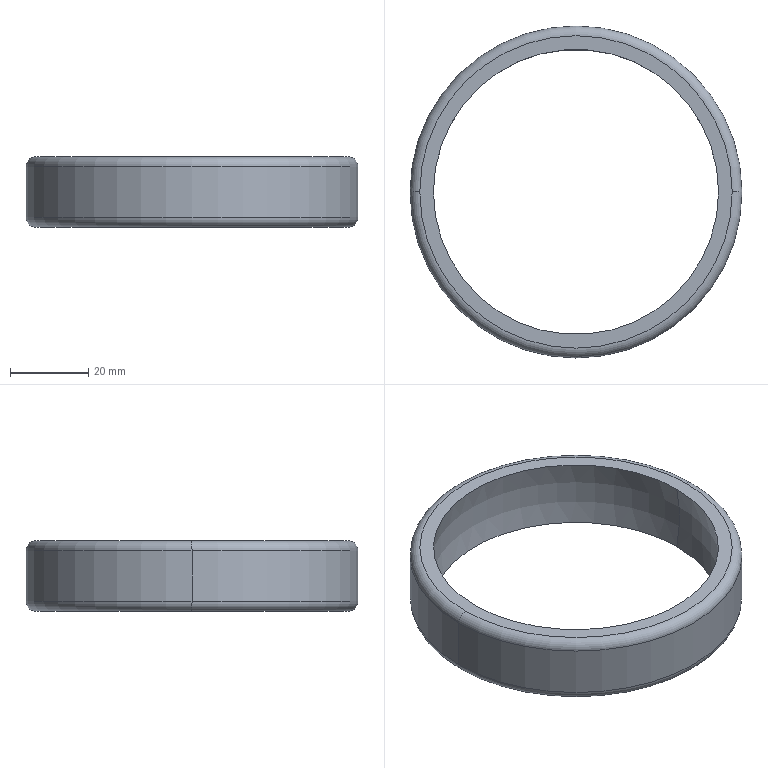Part | SolidWorks | features Extrusion 1, Fillet 1, RevCut 1 | 1 solid | 10 faces | box 85 x 85 x 18 mm | volume 23565 mm3 | torus 6 | cylinder 2 | plane 2 | commonest cylinder face diameters 85 x2
STEP:
#1=CARTESIAN_POINT('',(-40.,0.,-9.));
#2=VERTEX_POINT('',#1);
#3=CARTESIAN_POINT('',(40.,0.,-9.));
#4=VERTEX_POINT('',#3);
#5=CARTESIAN_POINT('',(0.,0.,-9.));
#6=DIRECTION('',(0.,0.,-1.));
#7=DIRECTION('',(1.,0.,0.));
#8=AXIS2_PLACEMENT_3D('',#5,#6,#7);
#9=CIRCLE('',#8,40.);
#10=EDGE_CURVE('',#2,#4,#9,.T.);
#11=ORIENTED_EDGE('',*,*,#10,.F.);
#12=CARTESIAN_POINT('',(-42.5,0.,-6.5));
#13=VERTEX_POINT('',#12);
#14=CARTESIAN_POINT('',(-40.,0.,-6.5));
#15=DIRECTION('',(0.,1.,0.));
#16=DIRECTION('',(-1.,0.,0.));
#17=AXIS2_PLACEMENT_3D('',#14,#15,#16);
#18=CIRCLE('',#17,2.5);
#19=EDGE_CURVE('',#2,#13,#18,.T.);
#20=ORIENTED_EDGE('',*,*,#19,.T.);
#21=CARTESIAN_POINT('',(42.5,0.,-6.5));
#22=VERTEX_POINT('',#21);
#23=CARTESIAN_POINT('',(0.,0.,-6.5));
#24=DIRECTION('',(0.,0.,1.));
#25=DIRECTION('',(1.,0.,0.));
#26=AXIS2_PLACEMENT_3D('',#23,#24,#25);
#27=CIRCLE('',#26,42.5);
#28=EDGE_CURVE('',#22,#13,#27,.T.);
#29=ORIENTED_EDGE('',*,*,#28,.F.);
#30=CARTESIAN_POINT('',(40.,0.,-6.5));
#31=DIRECTION('',(0.,-1.,0.));
#32=DIRECTION('',(0.,0.,-1.));
#33=AXIS2_PLACEMENT_3D('',#30,#31,#32);
#34=CIRCLE('',#33,2.5);
#35=EDGE_CURVE('',#4,#22,#34,.T.);
#36=ORIENTED_EDGE('',*,*,#35,.F.);
#37=EDGE_LOOP('',(#11,#20,#29,#36));
#38=FACE_OUTER_BOUND('',#37,.T.);
#39=CARTESIAN_POINT('',(0.,0.,-6.5));
#40=DIRECTION('',(0.,0.,1.));
#41=DIRECTION('',(1.,0.,0.));
#42=AXIS2_PLACEMENT_3D('',#39,#40,#41);
#43=TOROIDAL_SURFACE('',#42,40.,2.5);
#44=ADVANCED_FACE('',(#38),#43,.T.);
#45=CARTESIAN_POINT('',(-42.5,0.,6.5));
#46=VERTEX_POINT('',#45);
#47=CARTESIAN_POINT('',(42.5,0.,6.5));
#48=VERTEX_POINT('',#47);
#49=CARTESIAN_POINT('',(0.,0.,6.5));
#50=DIRECTION('',(0.,0.,-1.));
#51=DIRECTION('',(1.,0.,0.));
#52=AXIS2_PLACEMENT_3D('',#49,#50,#51);
#53=CIRCLE('',#52,42.5);
#54=EDGE_CURVE('',#46,#48,#53,.T.);
#55=ORIENTED_EDGE('',*,*,#54,.F.);
#56=CARTESIAN_POINT('',(-40.,0.,9.));
#57=VERTEX_POINT('',#56);
#58=CARTESIAN_POINT('',(-40.,0.,6.5));
#59=DIRECTION('',(0.,1.,0.));
#60=DIRECTION('',(-1.,0.,0.));
#61=AXIS2_PLACEMENT_3D('',#58,#59,#60);
#62=CIRCLE('',#61,2.5);
#63=EDGE_CURVE('',#46,#57,#62,.T.);
#64=ORIENTED_EDGE('',*,*,#63,.T.);
#65=CARTESIAN_POINT('',(40.,0.,9.));
#66=VERTEX_POINT('',#65);
#67=CARTESIAN_POINT('',(0.,0.,9.));
#68=DIRECTION('',(0.,0.,1.));
#69=DIRECTION('',(1.,0.,0.));
#70=AXIS2_PLACEMENT_3D('',#67,#68,#69);
#71=CIRCLE('',#70,40.);
#72=EDGE_CURVE('',#66,#57,#71,.T.);
#73=ORIENTED_EDGE('',*,*,#72,.F.);
#74=CARTESIAN_POINT('',(40.,0.,6.5));
#75=DIRECTION('',(0.,-1.,0.));
#76=DIRECTION('',(0.,0.,-1.));
#77=AXIS2_PLACEMENT_3D('',#74,#75,#76);
#78=CIRCLE('',#77,2.5);
#79=EDGE_CURVE('',#48,#66,#78,.T.);
#80=ORIENTED_EDGE('',*,*,#79,.F.);
#81=EDGE_LOOP('',(#55,#64,#73,#80));
#82=FACE_OUTER_BOUND('',#81,.T.);
#83=CARTESIAN_POINT('',(0.,0.,6.5));
#84=DIRECTION('',(0.,0.,1.));
#85=DIRECTION('',(1.,0.,0.));
#86=AXIS2_PLACEMENT_3D('',#83,#84,#85);
#87=TOROIDAL_SURFACE('',#86,40.,2.5);
#88=ADVANCED_FACE('',(#82),#87,.T.);
#89=CARTESIAN_POINT('',(36.5,0.,9.));
#90=VERTEX_POINT('',#89);
#91=CARTESIAN_POINT('',(-36.5,0.,9.));
#92=VERTEX_POINT('',#91);
#93=CARTESIAN_POINT('',(0.,0.,9.));
#94=DIRECTION('',(0.,0.,-1.));
#95=DIRECTION('',(-1.,0.,0.));
#96=AXIS2_PLACEMENT_3D('',#93,#94,#95);
#97=CIRCLE('',#96,36.5);
#98=EDGE_CURVE('',#90,#92,#97,.T.);
#99=ORIENTED_EDGE('',*,*,#98,.F.);
#100=CARTESIAN_POINT('',(36.5,0.,-9.));
#101=VERTEX_POINT('',#100);
#102=CARTESIAN_POINT('',(-7.591,0.,0.));
#103=DIRECTION('',(0.,1.,0.));
#104=DIRECTION('',(-1.,0.,0.));
#105=AXIS2_PLACEMENT_3D('',#102,#103,#104);
#106=CIRCLE('',#105,45.);
#107=EDGE_CURVE('',#90,#101,#106,.T.);
#108=ORIENTED_EDGE('',*,*,#107,.T.);
#109=CARTESIAN_POINT('',(-36.5,0.,-9.));
#110=VERTEX_POINT('',#109);
#111=CARTESIAN_POINT('',(0.,0.,-9.));
#112=DIRECTION('',(0.,0.,-1.));
#113=DIRECTION('',(-1.,0.,0.));
#114=AXIS2_PLACEMENT_3D('',#111,#112,#113);
#115=CIRCLE('',#114,36.5);
#116=EDGE_CURVE('',#101,#110,#115,.T.);
#117=ORIENTED_EDGE('',*,*,#116,.T.);
#118=CARTESIAN_POINT('',(7.591,0.,0.));
#119=DIRECTION('',(0.,-1.,0.));
#120=DIRECTION('',(0.,0.,-1.));
#121=AXIS2_PLACEMENT_3D('',#118,#119,#120);
#122=CIRCLE('',#121,45.);
#123=EDGE_CURVE('',#92,#110,#122,.T.);
#124=ORIENTED_EDGE('',*,*,#123,.F.);
#125=EDGE_LOOP('',(#99,#108,#117,#124));
#126=FACE_OUTER_BOUND('',#125,.T.);
#127=CARTESIAN_POINT('',(0.,0.,0.));
#128=DIRECTION('',(0.,0.,-1.));
#129=DIRECTION('',(-1.,0.,0.));
#130=AXIS2_PLACEMENT_3D('',#127,#128,#129);
#131=TOROIDAL_SURFACE('',#130,-7.591,45.);
#132=ADVANCED_FACE('',(#126),#131,.F.);
#133=ORIENTED_EDGE('',*,*,#54,.T.);
#134=CARTESIAN_POINT('',(42.5,0.,9.));
#135=DIRECTION('',(0.,0.,-1.));
#136=VECTOR('',#135,1000.);
#137=LINE('',#134,#136);
#138=EDGE_CURVE('',#48,#22,#137,.T.);
#139=ORIENTED_EDGE('',*,*,#138,.T.);
#140=ORIENTED_EDGE('',*,*,#28,.T.);
#141=CARTESIAN_POINT('',(-42.5,0.,9.));
#142=DIRECTION('',(0.,0.,-1.));
#143=VECTOR('',#142,1000.);
#144=LINE('',#141,#143);
#145=EDGE_CURVE('',#46,#13,#144,.T.);
#146=ORIENTED_EDGE('',*,*,#145,.F.);
#147=EDGE_LOOP('',(#133,#139,#140,#146));
#148=FACE_OUTER_BOUND('',#147,.T.);
#149=CARTESIAN_POINT('',(0.,0.,9.));
#150=DIRECTION('',(0.,0.,-1.));
#151=DIRECTION('',(-1.,0.,0.));
#152=AXIS2_PLACEMENT_3D('',#149,#150,#151);
#153=CYLINDRICAL_SURFACE('',#152,42.5);
#154=ADVANCED_FACE('',(#148),#153,.T.);
#155=ORIENTED_EDGE('',*,*,#72,.T.);
#156=CARTESIAN_POINT('',(0.,0.,9.));
#157=DIRECTION('',(0.,0.,1.));
#158=DIRECTION('',(1.,0.,0.));
#159=AXIS2_PLACEMENT_3D('',#156,#157,#158);
#160=CIRCLE('',#159,40.);
#161=EDGE_CURVE('',#57,#66,#160,.T.);
#162=ORIENTED_EDGE('',*,*,#161,.T.);
#163=EDGE_LOOP('',(#155,#162));
#164=FACE_OUTER_BOUND('',#163,.T.);
#165=CARTESIAN_POINT('',(0.,0.,9.));
#166=DIRECTION('',(0.,0.,-1.));
#167=DIRECTION('',(-1.,0.,0.));
#168=AXIS2_PLACEMENT_3D('',#165,#166,#167);
#169=CIRCLE('',#168,36.5);
#170=EDGE_CURVE('',#92,#90,#169,.T.);
#171=ORIENTED_EDGE('',*,*,#170,.T.);
#172=ORIENTED_EDGE('',*,*,#98,.T.);
#173=EDGE_LOOP('',(#171,#172));
#174=FACE_BOUND('',#173,.T.);
#175=CARTESIAN_POINT('',(0.,0.,9.));
#176=DIRECTION('',(0.,0.,1.));
#177=DIRECTION('',(1.,0.,0.));
#178=AXIS2_PLACEMENT_3D('',#175,#176,#177);
#179=PLANE('',#178);
#180=ADVANCED_FACE('',(#164,#174),#179,.T.);
#181=CARTESIAN_POINT('',(0.,0.,-9.));
#182=DIRECTION('',(0.,0.,-1.));
#183=DIRECTION('',(1.,0.,0.));
#184=AXIS2_PLACEMENT_3D('',#181,#182,#183);
#185=CIRCLE('',#184,40.);
#186=EDGE_CURVE('',#4,#2,#185,.T.);
#187=ORIENTED_EDGE('',*,*,#186,.T.);
#188=ORIENTED_EDGE('',*,*,#10,.T.);
#189=EDGE_LOOP('',(#187,#188));
#190=FACE_OUTER_BOUND('',#189,.T.);
#191=CARTESIAN_POINT('',(0.,0.,-9.));
#192=DIRECTION('',(0.,0.,-1.));
#193=DIRECTION('',(-1.,0.,0.));
#194=AXIS2_PLACEMENT_3D('',#191,#192,#193);
#195=CIRCLE('',#194,36.5);
#196=EDGE_CURVE('',#110,#101,#195,.T.);
#197=ORIENTED_EDGE('',*,*,#196,.F.);
#198=ORIENTED_EDGE('',*,*,#116,.F.);
#199=EDGE_LOOP('',(#197,#198));
#200=FACE_BOUND('',#199,.T.);
#201=CARTESIAN_POINT('',(0.,0.,-9.));
#202=DIRECTION('',(0.,0.,1.));
#203=DIRECTION('',(1.,0.,0.));
#204=AXIS2_PLACEMENT_3D('',#201,#202,#203);
#205=PLANE('',#204);
#206=ADVANCED_FACE('',(#190,#200),#205,.F.);
#207=ORIENTED_EDGE('',*,*,#138,.F.);
#208=CARTESIAN_POINT('',(0.,0.,6.5));
#209=DIRECTION('',(0.,0.,-1.));
#210=DIRECTION('',(1.,0.,0.));
#211=AXIS2_PLACEMENT_3D('',#208,#209,#210);
#212=CIRCLE('',#211,42.5);
#213=EDGE_CURVE('',#48,#46,#212,.T.);
#214=ORIENTED_EDGE('',*,*,#213,.T.);
#215=ORIENTED_EDGE('',*,*,#145,.T.);
#216=CARTESIAN_POINT('',(0.,0.,-6.5));
#217=DIRECTION('',(0.,0.,1.));
#218=DIRECTION('',(1.,0.,0.));
#219=AXIS2_PLACEMENT_3D('',#216,#217,#218);
#220=CIRCLE('',#219,42.5);
#221=EDGE_CURVE('',#13,#22,#220,.T.);
#222=ORIENTED_EDGE('',*,*,#221,.T.);
#223=EDGE_LOOP('',(#207,#214,#215,#222));
#224=FACE_OUTER_BOUND('',#223,.T.);
#225=CARTESIAN_POINT('',(0.,0.,9.));
#226=DIRECTION('',(0.,0.,-1.));
#227=DIRECTION('',(-1.,0.,0.));
#228=AXIS2_PLACEMENT_3D('',#225,#226,#227);
#229=CYLINDRICAL_SURFACE('',#228,42.5);
#230=ADVANCED_FACE('',(#224),#229,.T.);
#231=ORIENTED_EDGE('',*,*,#107,.F.);
#232=ORIENTED_EDGE('',*,*,#170,.F.);
#233=ORIENTED_EDGE('',*,*,#123,.T.);
#234=ORIENTED_EDGE('',*,*,#196,.T.);
#235=EDGE_LOOP('',(#231,#232,#233,#234));
#236=FACE_OUTER_BOUND('',#235,.T.);
#237=CARTESIAN_POINT('',(0.,0.,0.));
#238=DIRECTION('',(0.,0.,-1.));
#239=DIRECTION('',(-1.,0.,0.));
#240=AXIS2_PLACEMENT_3D('',#237,#238,#239);
#241=TOROIDAL_SURFACE('',#240,-7.591,45.);
#242=ADVANCED_FACE('',(#236),#241,.F.);
#243=ORIENTED_EDGE('',*,*,#63,.F.);
#244=ORIENTED_EDGE('',*,*,#213,.F.);
#245=ORIENTED_EDGE('',*,*,#79,.T.);
#246=ORIENTED_EDGE('',*,*,#161,.F.);
#247=EDGE_LOOP('',(#243,#244,#245,#246));
#248=FACE_OUTER_BOUND('',#247,.T.);
#249=CARTESIAN_POINT('',(0.,0.,6.5));
#250=DIRECTION('',(0.,0.,1.));
#251=DIRECTION('',(1.,0.,0.));
#252=AXIS2_PLACEMENT_3D('',#249,#250,#251);
#253=TOROIDAL_SURFACE('',#252,40.,2.5);
#254=ADVANCED_FACE('',(#248),#253,.T.);
#255=ORIENTED_EDGE('',*,*,#19,.F.);
#256=ORIENTED_EDGE('',*,*,#186,.F.);
#257=ORIENTED_EDGE('',*,*,#35,.T.);
#258=ORIENTED_EDGE('',*,*,#221,.F.);
#259=EDGE_LOOP('',(#255,#256,#257,#258));
#260=FACE_OUTER_BOUND('',#259,.T.);
#261=CARTESIAN_POINT('',(0.,0.,-6.5));
#262=DIRECTION('',(0.,0.,1.));
#263=DIRECTION('',(1.,0.,0.));
#264=AXIS2_PLACEMENT_3D('',#261,#262,#263);
#265=TOROIDAL_SURFACE('',#264,40.,2.5);
#266=ADVANCED_FACE('',(#260),#265,.T.);
#267=CLOSED_SHELL('',(#44,#88,#132,#154,#180,#206,#230,#242,#254,#266));
#268=MANIFOLD_SOLID_BREP('',#267);
#269=CARTESIAN_POINT('',(0.,0.,0.));
#270=DIRECTION('',(0.,0.,1.));
#271=DIRECTION('',(1.,0.,0.));
#272=AXIS2_PLACEMENT_3D('',#269,#270,#271);
#273=(LENGTH_UNIT()NAMED_UNIT(*)SI_UNIT(.MILLI.,.METRE.));
#274=UNCERTAINTY_MEASURE_WITH_UNIT(LENGTH_MEASURE(0.00001),#273,'','');
#275=(NAMED_UNIT(*)PLANE_ANGLE_UNIT()SI_UNIT($,.RADIAN.));
#276=(NAMED_UNIT(*)SI_UNIT($,.STERADIAN.)SOLID_ANGLE_UNIT());
#277=(GEOMETRIC_REPRESENTATION_CONTEXT(3)GLOBAL_UNCERTAINTY_ASSIGNED_CONTEXT((#274))GLOBAL_UNIT_ASSIGNED_CONTEXT((#273,#275,#276))REPRESENTATION_CONTEXT('',''));
#278=ADVANCED_BREP_SHAPE_REPRESENTATION('',(#268,#272),#277);